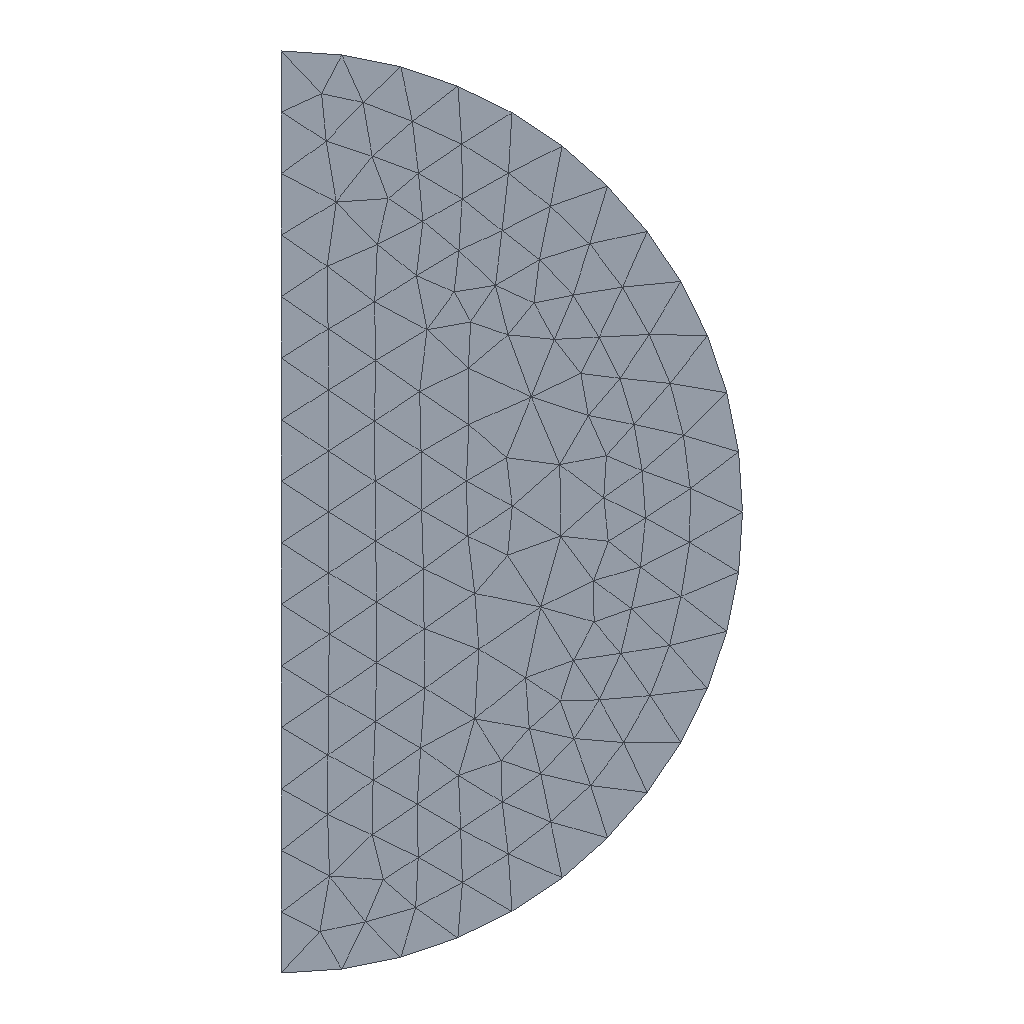Simulation study | comsol
Notes in the study folder:
k_Nb 52.335[W/(m*K)] Thermal conductivity Nb
rho_Nb 8.57e3[kg/m^3] Density Nb
Cp_Nb 2.7e2[J/(kg*K)] Heat capacity Nb
T_0 2.7315e2[K] Initial temperature
T_appl 1.27315e3[K] Boundary temperature
Set-up summary:
category,name,step,type,value,unit,region
solver,comsol,,COMSOL Multiphysics 6.4 (Build: 293)
units,SI; geometry length unit m,,stated,COMSOL default unit system (SI)
analysis,Study 1,,Transient,space_dimension=2D
load_step,std1/time,std1/time,Transient,"type=Transient; times=range(0,2,300)"
mesh,nodes,,,154
mesh,elements,,,267
element_type,tri,,,267
element_type,edg,,,39
element_type,vtx,,,3
component,mod1,,2D,geometry=geom1; domains=1
physics,Heat Transfer (ht),mod1,HeatTransfer,"T(T), discontinuousdamagedtissueindicator(discontinuousdamagedtissueindicator), continuousdamagedtissueindicator(continuousdamagedtissueindicator), thermaldamageindicator(thermaldamageindicator), radiativeintensity(radiativeintensity), incidentradiation(incidentradiation), surfaceradiosity(surfaceradiosity)"
parameter,k_Nb,,,52.335[W/(m*K)]
parameter,rho_Nb,,,8.57e3[kg/m^3]
parameter,Cp_Nb,,,2.7e2[J/(kg*K)]
parameter,T_0,,,2.7315e2[K]
parameter,T_appl,,,1.27315e3[K]
bc,Heat Transfer in Solids 1 (solid1),mod1/ht,SolidHeatTransferModel,k=k_Nb; rho=rho_Nb; Cp=Cp_Nb; streamline=0; crosswind=0; pref=1[atm]; hasPhaseChange=0; Solid_material=dommat; u_prime=0 0 0; dfltopaque=1; thermalConductivityModel=Standard,,selection [1]
bc,Axial Symmetry 1 (axi1),mod1/ht,AxialSymmetry,,,selection [1]
bc,Thermal Insulation 1 (ins1),mod1/ht,ThermalInsulation,,,selection []
bc,Initial Values 1 (init1),mod1/ht,init,Tinit=T_0; Tinit_resistive=293.15[K],,selection [1]
bc,Continuity (dcont1),mod1/ht,Continuity,pairDisconnect=1; pairSelection=all; pairsList=0,,selection []
bc,Temperature 1 (temp1),mod1/ht,TemperatureBoundary,T0=T_appl,,"selection [2, 3]"
bc,Local Thermal Nonequilibrium Boundary 1 (ltneb1),mod1/ht,LocalThermalNonequilibriumBoundary,,,selection []
COMSOL model file for Java, long lists of numbers shortened:
/*
 * em_deck.java
 */

import com.comsol.model.*;
import com.comsol.model.util.*;

/** Model exported on Oct 28 2026, 10:37 by COMSOL 6.4.0.293. */
public class em_deck {

  public static Model run() {
    Model model = ModelUtil.create("Model");

    model.modelPath("");

    model.label("in.mph");

    model.param().set("k_Nb", "52.335[W/(m*K)]", "Thermal conductivity Nb");
    model.param().set("rho_Nb", "8.57e3[kg/m^3]", "Density Nb");
    model.param().set("Cp_Nb", "2.7e2[J/(kg*K)]", "Heat capacity Nb");
    model.param().set("T_0", "2.7315e2[K]", "Initial temperature");
    model.param().set("T_appl", "1.27315e3[K]", "Boundary temperature");

    model.component().create("mod1", false);

    model.component("mod1").geom().create("geom1", 2);

    model.component("mod1").label("Model 1");

    model.component("mod1").defineLocalCoord(false);

    model.component("mod1").curvedInterior(false);

    model.component("mod1").geom("geom1").axisymmetric(true);

    model.component("mod1").mesh().create("mesh1");

    model.component("mod1").geom("geom1").repairTolType("relative");
    model.component("mod1").geom("geom1").create("c1", "Circle");
    model.component("mod1").geom("geom1").feature("c1").set("r", 0.4);
    model.component("mod1").geom("geom1").create("r1", "Rectangle");
    model.component("mod1").geom("geom1").feature("r1").set("size", new double[]{0.4, 0.8});
    model.component("mod1").geom("geom1").feature("r1").set("pos", new double[]{-0.4, -0.4});
    model.component("mod1").geom("geom1").create("dif1", "Difference");
    model.component("mod1").geom("geom1").feature("dif1").selection("input").set("c1");
    model.component("mod1").geom("geom1").feature("dif1").selection("input2").set("r1");
    model.component("mod1").geom("geom1").feature("fin").set("repairtoltype", "relative");
    model.component("mod1").geom("geom1").run();

    model.view().create("view2", 3);
    model.view("view2").light().create("lgt4", "DirectionalLight");

    model.component("mod1").physics().create("ht", "HeatTransfer", "geom1");
    model.component("mod1").physics("ht").create("temp1", "TemperatureBoundary", 1);
    model.component("mod1").physics("ht").feature("temp1").selection().set(2, 3);

    model.component("mod1").mesh("mesh1").create("ftri1", "FreeTri");

    model.thermodynamics().label("Thermodynamics Package");

    model.component("mod1").view("view1").set("showlabels", true);
    model.component("mod1").view("view1").axis().set("xmin", -0.06358);
    model.component("mod1").view("view1").axis().set("xmax", 0.4636);
    model.component("mod1").view("view1").axis().set("ymin", -0.44);
    model.component("mod1").view("view1").axis().set("ymax", 0.44);
    model.view("view2").light("lgt1").set("lightdirection", "-(-1) -(1) -(-1) ");
    model.view("view2").light("lgt1").set("intensity", 0.5);
    model.view("view2").light("lgt1").set("cameracoord", false);
    model.view("view2").light("lgt2").set("lightdirection", "-(1) -(-1) -(1) ");
    model.view("view2").light("lgt2").set("intensity", 0.5);
    model.view("view2").light("lgt2").set("cameracoord", false);
    model.view("view2").light("lgt3").set("lightdirection", "-(1) -(1) -(-1) ");
    model.view("view2").light("lgt3").set("intensity", 0.5);
    model.view("view2").light("lgt3").set("cameracoord", false);
    model.view("view2").light("lgt3").set("castshadowsonfloor", false);
    model.view("view2").light("lgt4").set("lightdirection", "-(-1) -(-1) -(1) ");
    model.view("view2").light("lgt4").set("castshadowsonfloor", true);

    model.component("mod1").physics("ht").label("Heat Transfer");
    model.component("mod1").physics("ht").prop("ShapeProperty").set("boundaryFlux_temperature", false);
    model.component("mod1").physics("ht").prop("PhysicalModelProperty").set("BackCompStateT", 0);
    model.component("mod1").physics("ht").prop("ConsistentStabilization").set("heatCrosswindDiffusion", false);
    model.component("mod1").physics("ht").prop("ConsistentStabilization").set("StreamlineDiffusionOldForm", true);
    model.component("mod1").physics("ht").prop("ParticipatingMediaSettingsProperty").set("PerfIndex", 0.5);
    model.component("mod1").physics("ht").prop("RadiationSettings").set("lambda_r", "(0)/1[um]");
    model.component("mod1").physics("ht").feature("solid1").set("k_mat", "userdef");
    model.component("mod1").physics("ht").feature("solid1")
         .set("k", new String[][]{{"k_Nb"}, {"0"}, {"0"}, {"0"}, {"k_Nb"}, {"0"}, {"0"}, {"0"}, {"k_Nb"}});
    model.component("mod1").physics("ht").feature("solid1").set("rho_mat", "userdef");
    model.component("mod1").physics("ht").feature("solid1").set("rho", "rho_Nb");
    model.component("mod1").physics("ht").feature("solid1").set("Cp_mat", "userdef");
    model.component("mod1").physics("ht").feature("solid1").set("Cp", "Cp_Nb");
    model.component("mod1").physics("ht").feature("solid1").set("minput_temperature_src", "root.mod1.T");
    model.component("mod1").physics("ht").feature("solid1").set("minput_strainreferencetemperature_src", "userdef");
    model.component("mod1").physics("ht").feature("solid1").set("minput_strainreferencetemperature", 0);
    model.component("mod1").physics("ht").feature("solid1").label("Heat Transfer in Solids 1");
    model.component("mod1").physics("ht").feature("init1").set("Tinit", "T_0");
    model.component("mod1").physics("ht").feature("dcont1").set("pairDisconnect", true);
    model.component("mod1").physics("ht").feature("dcont1").label("Continuity");
    model.component("mod1").physics("ht").feature("temp1").set("T0", "T_appl");

    model.component("mod1").mesh("mesh1").feature("ftri1").set("smoothcontrol", true);
    model.component("mod1").mesh("mesh1").feature("ftri1").set("smoothmaxiter", 8);
    model.component("mod1").mesh("mesh1").feature("ftri1").set("smoothmaxdepth", 8);
    model.component("mod1").mesh("mesh1").run();

    model.study().create("std1");
    model.study("std1").create("time", "Transient");

    model.sol().create("sol1");
    model.sol("sol1").attach("std1");
    model.sol("sol1").create("st1", "StudyStep");
    model.sol("sol1").create("v1", "Variables");
    model.sol("sol1").create("t1", "Time");
    model.sol("sol1").feature("t1").create("fc1", "FullyCoupled");
    model.sol("sol1").feature("t1").create("d1", "Direct");
    model.sol("sol1").feature("t1").feature().remove("fcDef");

    model.result().dataset().create("rev1", "Revolve2D");
    model.result().create("pg1", "PlotGroup2D");
    model.result().create("pg2", "PlotGroup3D");
    model.result("pg1").create("surf1", "Surface");
    model.result("pg2").create("surf1", "Surface");
    model.result("pg2").feature("surf1").set("data", "rev1");

    model.study("std1").feature("time").set("tlist", "range(0,2,300)");

    model.sol("sol1").label("Solver 1");
    model.sol("sol1").feature("st1").label("Compile Equations: Time Dependent");
    model.sol("sol1").feature("v1").label("Dependent Variables 1.1");
    model.sol("sol1").feature("v1").set("clistctrl", new String[]{});
    model.sol("sol1").feature("v1").set("cname", new String[]{});
    model.sol("sol1").feature("v1").set("clist", new int[]{});
    model.sol("sol1").feature("t1").label("Time-Dependent Solver 1.1");
    model.sol("sol1").feature("t1").set("tlist", "range(0,2,300)");
    model.sol("sol1").feature("t1").set("atolglobalvaluemethod", "manual");
    model.sol("sol1").feature("t1").set("atolglobal", "0.001");
    model.sol("sol1").feature("t1").set("ewtrescale", false);
    model.sol("sol1").feature("t1").set("atolvaluemethod", new String[]{"mod1_T", "manual"});
    model.sol("sol1").feature("t1").set("initialstepbdf", "0.001");
    model.sol("sol1").feature("t1").set("maxorder", 2);
    model.sol("sol1").feature("t1").set("bwinitstepfrac", "1.0");
    model.sol("sol1").feature("t1").set("estrat", "exclude");
    model.sol("sol1").feature("t1").feature("dDef").label("Direct 2");
    model.sol("sol1").feature("t1").feature("dDef").set("thresh", 0.1);
    model.sol("sol1").feature("t1").feature("dDef").set("ooc", false);
    model.sol("sol1").feature("t1").feature("dDef").set("rhob", 400);
    model.sol("sol1").feature("t1").feature("aDef").label("Advanced 1");
    model.sol("sol1").feature("t1").feature("fc1").label("Fully Coupled 1.1");
    model.sol("sol1").feature("t1").feature("fc1").set("maxiter", 5);
    model.sol("sol1").feature("t1").feature("fc1").set("jtech", "once");
    model.sol("sol1").feature("t1").feature("fc1").set("probesel", "manual");
    model.sol("sol1").feature("t1").feature("d1").label("Direct 1.1");
    model.sol("sol1").feature("t1").feature("d1").set("linsolver", "pardiso");
    model.sol("sol1").feature("t1").feature("d1").set("ooc", false);
    model.sol("sol1").feature("t1").feature("d1").set("pardreorder", "ndmt");
    model.sol("sol1").feature("t1").feature("d1").set("pivotstrategy", false);
    model.sol("sol1").feature("t1").feature("d1").set("rhob", 400);

    model.study("std1").runNoGen();

    model.result().dataset("dset1").label("Solution 1");
    model.result().dataset("rev1").set("genpoints", new double[][]{{0, 0}, {0, 0.4}});
    model.result().dataset("rev1").set("layermethod", "custom");
    model.result().dataset("rev1").set("revangle", 180);
    model.result().dataset("rev1").set("planemap", "xy");
    model.result("pg1").set("smooth", "internal");
    model.result("pg1").feature("surf1").set("unit", "degC");
    model.result("pg1").feature("surf1").set("colortable", "RainbowClassic");
    model.result("pg1").feature("surf1").set("smooth", "internal");
    model.result("pg1").feature("surf1").set("resolution", "normal");
    model.result("pg2").set("smooth", "internal");
    model.result("pg2").feature("surf1").set("unit", "degC");
    model.result("pg2").feature("surf1").set("colortable", "RainbowClassic");
    model.result("pg2").feature("surf1").set("smooth", "internal");
    model.result("pg2").feature("surf1").set("resolution", "normal");

    return model;
  }

  public static void main(String[] args) {
    run();
  }

}
Results summary:
result,max T = abs(mod1.T),dset1 (151 solution(s)),,1273.15,K